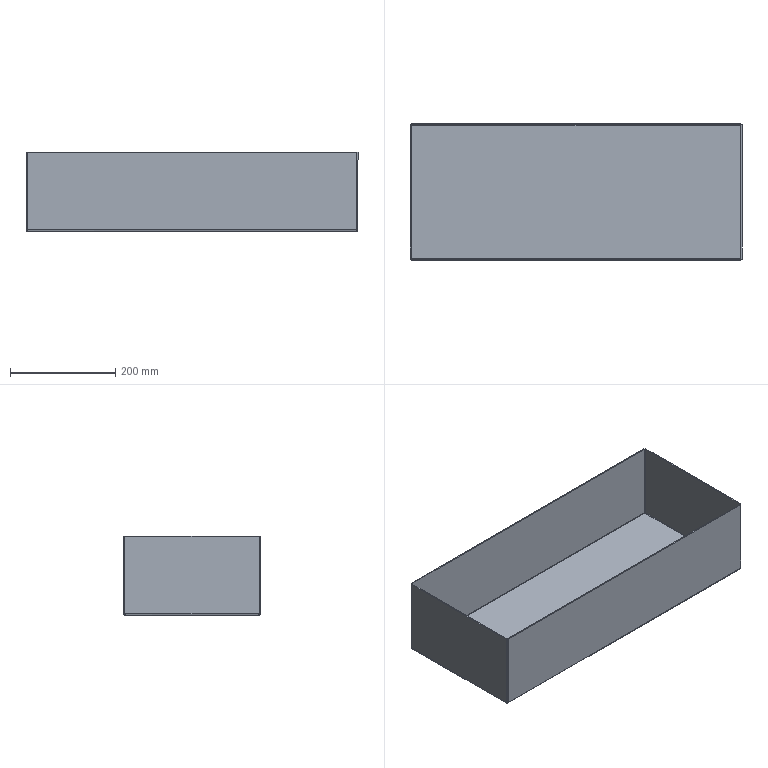Part | SolidWorks | features EdgeFlange 1, FlatPattern 1, SMBaseFlange 1, SheetMetal 1 | 1 solid | 38 faces | box 630 x 260 x 150 mm | volume 844986 mm3 | plane 22 | spline 8 | cylinder 8 | commonest cylinder face diameters 2 x4 6 x4
STEP:
#1=CARTESIAN_POINT('',(312.,127.,-2.));
#2=VERTEX_POINT('',#1);
#3=CARTESIAN_POINT('',(312.,-127.,-2.));
#4=VERTEX_POINT('',#3);
#5=CARTESIAN_POINT('',(312.,127.293,-2.));
#6=DIRECTION('',(0.,-1.,0.));
#7=VECTOR('',#6,1000.);
#8=LINE('',#5,#7);
#9=EDGE_CURVE('',#2,#4,#8,.T.);
#10=ORIENTED_EDGE('',*,*,#9,.T.);
#11=CARTESIAN_POINT('',(-312.,-127.,-2.));
#12=VERTEX_POINT('',#11);
#13=CARTESIAN_POINT('',(312.293,-127.,-2.));
#14=DIRECTION('',(-1.,0.,0.));
#15=VECTOR('',#14,1000.);
#16=LINE('',#13,#15);
#17=EDGE_CURVE('',#4,#12,#16,.T.);
#18=ORIENTED_EDGE('',*,*,#17,.T.);
#19=CARTESIAN_POINT('',(-312.,127.,-2.));
#20=VERTEX_POINT('',#19);
#21=CARTESIAN_POINT('',(-312.,-127.293,-2.));
#22=DIRECTION('',(0.,1.,0.));
#23=VECTOR('',#22,1000.);
#24=LINE('',#21,#23);
#25=EDGE_CURVE('',#12,#20,#24,.T.);
#26=ORIENTED_EDGE('',*,*,#25,.T.);
#27=CARTESIAN_POINT('',(-312.293,127.,-2.));
#28=DIRECTION('',(1.,0.,0.));
#29=VECTOR('',#28,1000.);
#30=LINE('',#27,#29);
#31=EDGE_CURVE('',#20,#2,#30,.T.);
#32=ORIENTED_EDGE('',*,*,#31,.T.);
#33=EDGE_LOOP('',(#10,#18,#26,#32));
#34=FACE_OUTER_BOUND('',#33,.T.);
#35=CARTESIAN_POINT('',(0.,0.,-2.));
#36=DIRECTION('',(0.,0.,1.));
#37=DIRECTION('',(1.,0.,0.));
#38=AXIS2_PLACEMENT_3D('',#35,#36,#37);
#39=PLANE('',#38);
#40=ADVANCED_FACE('',(#34),#39,.F.);
#41=CARTESIAN_POINT('',(312.,-127.,0.));
#42=VERTEX_POINT('',#41);
#43=CARTESIAN_POINT('',(-312.,-127.,0.));
#44=VERTEX_POINT('',#43);
#45=CARTESIAN_POINT('',(312.293,-127.,0.));
#46=DIRECTION('',(-1.,0.,0.));
#47=VECTOR('',#46,1000.);
#48=LINE('',#45,#47);
#49=EDGE_CURVE('',#42,#44,#48,.T.);
#50=ORIENTED_EDGE('',*,*,#49,.F.);
#51=CARTESIAN_POINT('',(312.,127.,0.));
#52=VERTEX_POINT('',#51);
#53=CARTESIAN_POINT('',(312.,127.293,0.));
#54=DIRECTION('',(0.,-1.,0.));
#55=VECTOR('',#54,1000.);
#56=LINE('',#53,#55);
#57=EDGE_CURVE('',#52,#42,#56,.T.);
#58=ORIENTED_EDGE('',*,*,#57,.F.);
#59=CARTESIAN_POINT('',(-312.,127.,0.));
#60=VERTEX_POINT('',#59);
#61=CARTESIAN_POINT('',(-312.293,127.,0.));
#62=DIRECTION('',(1.,0.,0.));
#63=VECTOR('',#62,1000.);
#64=LINE('',#61,#63);
#65=EDGE_CURVE('',#60,#52,#64,.T.);
#66=ORIENTED_EDGE('',*,*,#65,.F.);
#67=CARTESIAN_POINT('',(-312.,-127.293,0.));
#68=DIRECTION('',(0.,1.,0.));
#69=VECTOR('',#68,1000.);
#70=LINE('',#67,#69);
#71=EDGE_CURVE('',#44,#60,#70,.T.);
#72=ORIENTED_EDGE('',*,*,#71,.F.);
#73=EDGE_LOOP('',(#50,#58,#66,#72));
#74=FACE_OUTER_BOUND('',#73,.T.);
#75=CARTESIAN_POINT('',(0.,0.,0.));
#76=DIRECTION('',(0.,0.,1.));
#77=DIRECTION('',(1.,0.,0.));
#78=AXIS2_PLACEMENT_3D('',#75,#76,#77);
#79=PLANE('',#78);
#80=ADVANCED_FACE('',(#74),#79,.T.);
#81=CARTESIAN_POINT('',(-315.,127.293,1.));
#82=VERTEX_POINT('',#81);
#83=CARTESIAN_POINT('',(-313.,127.293,1.));
#84=VERTEX_POINT('',#83);
#85=CARTESIAN_POINT('',(-313.,127.293,1.));
#86=DIRECTION('',(1.,0.,0.));
#87=VECTOR('',#86,1000.);
#88=LINE('',#85,#87);
#89=EDGE_CURVE('',#82,#84,#88,.T.);
#90=ORIENTED_EDGE('',*,*,#89,.T.);
#91=CARTESIAN_POINT('',(-312.,127.,0.));
#92=CARTESIAN_POINT('',(-312.262,127.049,0.));
#93=CARTESIAN_POINT('',(-312.522,127.098,0.1078));
#94=CARTESIAN_POINT('',(-312.892,127.195,0.478));
#95=CARTESIAN_POINT('',(-313.,127.244,0.7382));
#96=CARTESIAN_POINT('',(-313.,127.293,1.));
#97=B_SPLINE_CURVE_WITH_KNOTS('',3,(#91,#92,#93,#94,#95,#96),.UNSPECIFIED.,.F.,.F.,(4,2,4),(0.,0.5,1.),.UNSPECIFIED.);
#98=EDGE_CURVE('',#60,#84,#97,.T.);
#99=ORIENTED_EDGE('',*,*,#98,.F.);
#100=CARTESIAN_POINT('',(-312.,127.,0.));
#101=DIRECTION('',(0.,0.,-1.));
#102=VECTOR('',#101,1000.);
#103=LINE('',#100,#102);
#104=EDGE_CURVE('',#60,#20,#103,.T.);
#105=ORIENTED_EDGE('',*,*,#104,.T.);
#106=CARTESIAN_POINT('',(-312.,127.,-2.));
#107=CARTESIAN_POINT('',(-312.393,127.024,-2.));
#108=CARTESIAN_POINT('',(-312.785,127.049,-1.922));
#109=CARTESIAN_POINT('',(-313.511,127.098,-1.621));
#110=CARTESIAN_POINT('',(-313.844,127.122,-1.399));
#111=CARTESIAN_POINT('',(-314.399,127.171,-0.8436));
#112=CARTESIAN_POINT('',(-314.621,127.195,-0.5109));
#113=CARTESIAN_POINT('',(-314.922,127.244,0.2148));
#114=CARTESIAN_POINT('',(-315.,127.268,0.6073));
#115=CARTESIAN_POINT('',(-315.,127.293,1.));
#116=B_SPLINE_CURVE_WITH_KNOTS('',3,(#106,#107,#108,#109,#110,#111,#112,#113,#114,#115),.UNSPECIFIED.,.F.,.F.,(4,2,2,2,4),(0.,0.25,0.5,0.75,1.),.UNSPECIFIED.);
#117=EDGE_CURVE('',#20,#82,#116,.T.);
#118=ORIENTED_EDGE('',*,*,#117,.T.);
#119=EDGE_LOOP('',(#90,#99,#105,#118));
#120=FACE_OUTER_BOUND('',#119,.T.);
#121=CARTESIAN_POINT('',(-312.,127.,-2.02));
#122=CARTESIAN_POINT('',(-312.395,127.024,-2.02));
#123=CARTESIAN_POINT('',(-312.79,127.049,-1.941));
#124=CARTESIAN_POINT('',(-313.521,127.098,-1.639));
#125=CARTESIAN_POINT('',(-313.856,127.122,-1.415));
#126=CARTESIAN_POINT('',(-314.415,127.171,-0.8559));
#127=CARTESIAN_POINT('',(-314.639,127.195,-0.5209));
#128=CARTESIAN_POINT('',(-314.941,127.244,0.2095));
#129=CARTESIAN_POINT('',(-315.02,127.268,0.6046));
#130=CARTESIAN_POINT('',(-315.02,127.293,1.));
#131=CARTESIAN_POINT('',(-312.,127.,-2.));
#132=CARTESIAN_POINT('',(-312.393,127.024,-2.));
#133=CARTESIAN_POINT('',(-312.785,127.049,-1.922));
#134=CARTESIAN_POINT('',(-313.511,127.098,-1.621));
#135=CARTESIAN_POINT('',(-313.844,127.122,-1.399));
#136=CARTESIAN_POINT('',(-314.399,127.171,-0.8436));
#137=CARTESIAN_POINT('',(-314.621,127.195,-0.5109));
#138=CARTESIAN_POINT('',(-314.922,127.244,0.2148));
#139=CARTESIAN_POINT('',(-315.,127.268,0.6072));
#140=CARTESIAN_POINT('',(-315.,127.293,1.));
#141=CARTESIAN_POINT('',(-312.,127.,0.));
#142=CARTESIAN_POINT('',(-312.131,127.024,0.));
#143=CARTESIAN_POINT('',(-312.262,127.049,0.02603));
#144=CARTESIAN_POINT('',(-312.504,127.098,0.1262));
#145=CARTESIAN_POINT('',(-312.615,127.122,0.2003));
#146=CARTESIAN_POINT('',(-312.8,127.171,0.3855));
#147=CARTESIAN_POINT('',(-312.874,127.195,0.4964));
#148=CARTESIAN_POINT('',(-312.974,127.244,0.7383));
#149=CARTESIAN_POINT('',(-313.,127.268,0.8691));
#150=CARTESIAN_POINT('',(-313.,127.293,1.));
#151=CARTESIAN_POINT('',(-312.,127.,0.0202));
#152=CARTESIAN_POINT('',(-312.128,127.024,0.0202));
#153=CARTESIAN_POINT('',(-312.256,127.049,0.0457));
#154=CARTESIAN_POINT('',(-312.493,127.098,0.1439));
#155=CARTESIAN_POINT('',(-312.602,127.122,0.2165));
#156=CARTESIAN_POINT('',(-312.784,127.171,0.3979));
#157=CARTESIAN_POINT('',(-312.856,127.195,0.5066));
#158=CARTESIAN_POINT('',(-312.954,127.244,0.7435));
#159=CARTESIAN_POINT('',(-312.98,127.268,0.8717));
#160=CARTESIAN_POINT('',(-312.98,127.293,1.));
#161=B_SPLINE_SURFACE_WITH_KNOTS('',1,3,((#121,#122,#123,#124,#125,#126,#127,#128,#129,#130),(#131,#132,#133,#134,#135,#136,#137,#138,#139,#140),(#141,#142,#143,#144,#145,#146,#147,#148,#149,#150),(#151,#152,#153,#154,#155,#156,#157,#158,#159,#160)),.UNSPECIFIED.,.F.,.F.,.F.,(2,1,1,2),(4,2,2,2,4),(-0.01,0.,1.,1.01),(0.,0.25,0.5,0.75,1.),.UNSPECIFIED.);
#162=ADVANCED_FACE('',(#120),#161,.F.);
#163=CARTESIAN_POINT('',(-313.,-127.293,1.));
#164=VERTEX_POINT('',#163);
#165=CARTESIAN_POINT('',(-313.,-127.293,1.));
#166=CARTESIAN_POINT('',(-313.,-127.244,0.7382));
#167=CARTESIAN_POINT('',(-312.892,-127.195,0.478));
#168=CARTESIAN_POINT('',(-312.522,-127.098,0.1078));
#169=CARTESIAN_POINT('',(-312.262,-127.049,0.));
#170=CARTESIAN_POINT('',(-312.,-127.,0.));
#171=B_SPLINE_CURVE_WITH_KNOTS('',3,(#165,#166,#167,#168,#169,#170),.UNSPECIFIED.,.F.,.F.,(4,2,4),(0.,0.5,1.),.UNSPECIFIED.);
#172=EDGE_CURVE('',#164,#44,#171,.T.);
#173=ORIENTED_EDGE('',*,*,#172,.F.);
#174=CARTESIAN_POINT('',(-315.,-127.293,1.));
#175=VERTEX_POINT('',#174);
#176=CARTESIAN_POINT('',(-313.,-127.293,1.));
#177=DIRECTION('',(1.,0.,0.));
#178=VECTOR('',#177,1000.);
#179=LINE('',#176,#178);
#180=EDGE_CURVE('',#175,#164,#179,.T.);
#181=ORIENTED_EDGE('',*,*,#180,.F.);
#182=CARTESIAN_POINT('',(-315.,-127.293,1.));
#183=CARTESIAN_POINT('',(-315.,-127.268,0.6073));
#184=CARTESIAN_POINT('',(-314.922,-127.244,0.2148));
#185=CARTESIAN_POINT('',(-314.621,-127.195,-0.5109));
#186=CARTESIAN_POINT('',(-314.399,-127.171,-0.8436));
#187=CARTESIAN_POINT('',(-313.844,-127.122,-1.399));
#188=CARTESIAN_POINT('',(-313.511,-127.098,-1.621));
#189=CARTESIAN_POINT('',(-312.785,-127.049,-1.922));
#190=CARTESIAN_POINT('',(-312.393,-127.024,-2.));
#191=CARTESIAN_POINT('',(-312.,-127.,-2.));
#192=B_SPLINE_CURVE_WITH_KNOTS('',3,(#182,#183,#184,#185,#186,#187,#188,#189,#190,#191),.UNSPECIFIED.,.F.,.F.,(4,2,2,2,4),(0.,0.25,0.5,0.75,1.),.UNSPECIFIED.);
#193=EDGE_CURVE('',#175,#12,#192,.T.);
#194=ORIENTED_EDGE('',*,*,#193,.T.);
#195=CARTESIAN_POINT('',(-312.,-127.,0.));
#196=DIRECTION('',(0.,0.,-1.));
#197=VECTOR('',#196,1000.);
#198=LINE('',#195,#197);
#199=EDGE_CURVE('',#44,#12,#198,.T.);
#200=ORIENTED_EDGE('',*,*,#199,.F.);
#201=EDGE_LOOP('',(#173,#181,#194,#200));
#202=FACE_OUTER_BOUND('',#201,.T.);
#203=CARTESIAN_POINT('',(-315.02,-127.293,1.));
#204=CARTESIAN_POINT('',(-315.02,-127.268,0.6046));
#205=CARTESIAN_POINT('',(-314.941,-127.244,0.2095));
#206=CARTESIAN_POINT('',(-314.639,-127.195,-0.5209));
#207=CARTESIAN_POINT('',(-314.415,-127.171,-0.8559));
#208=CARTESIAN_POINT('',(-313.856,-127.122,-1.415));
#209=CARTESIAN_POINT('',(-313.521,-127.098,-1.639));
#210=CARTESIAN_POINT('',(-312.79,-127.049,-1.941));
#211=CARTESIAN_POINT('',(-312.395,-127.024,-2.02));
#212=CARTESIAN_POINT('',(-312.,-127.,-2.02));
#213=CARTESIAN_POINT('',(-315.,-127.293,1.));
#214=CARTESIAN_POINT('',(-315.,-127.268,0.6072));
#215=CARTESIAN_POINT('',(-314.922,-127.244,0.2148));
#216=CARTESIAN_POINT('',(-314.621,-127.195,-0.5109));
#217=CARTESIAN_POINT('',(-314.399,-127.171,-0.8436));
#218=CARTESIAN_POINT('',(-313.844,-127.122,-1.399));
#219=CARTESIAN_POINT('',(-313.511,-127.098,-1.621));
#220=CARTESIAN_POINT('',(-312.785,-127.049,-1.922));
#221=CARTESIAN_POINT('',(-312.393,-127.024,-2.));
#222=CARTESIAN_POINT('',(-312.,-127.,-2.));
#223=CARTESIAN_POINT('',(-313.,-127.293,1.));
#224=CARTESIAN_POINT('',(-313.,-127.268,0.8691));
#225=CARTESIAN_POINT('',(-312.974,-127.244,0.7383));
#226=CARTESIAN_POINT('',(-312.874,-127.195,0.4964));
#227=CARTESIAN_POINT('',(-312.8,-127.171,0.3855));
#228=CARTESIAN_POINT('',(-312.615,-127.122,0.2003));
#229=CARTESIAN_POINT('',(-312.504,-127.098,0.1262));
#230=CARTESIAN_POINT('',(-312.262,-127.049,0.02603));
#231=CARTESIAN_POINT('',(-312.131,-127.024,0.));
#232=CARTESIAN_POINT('',(-312.,-127.,0.));
#233=CARTESIAN_POINT('',(-312.98,-127.293,1.));
#234=CARTESIAN_POINT('',(-312.98,-127.268,0.8717));
#235=CARTESIAN_POINT('',(-312.954,-127.244,0.7435));
#236=CARTESIAN_POINT('',(-312.856,-127.195,0.5066));
#237=CARTESIAN_POINT('',(-312.784,-127.171,0.3979));
#238=CARTESIAN_POINT('',(-312.602,-127.122,0.2165));
#239=CARTESIAN_POINT('',(-312.493,-127.098,0.1439));
#240=CARTESIAN_POINT('',(-312.256,-127.049,0.0457));
#241=CARTESIAN_POINT('',(-312.128,-127.024,0.0202));
#242=CARTESIAN_POINT('',(-312.,-127.,0.0202));
#243=B_SPLINE_SURFACE_WITH_KNOTS('',1,3,((#203,#204,#205,#206,#207,#208,#209,#210,#211,#212),(#213,#214,#215,#216,#217,#218,#219,#220,#221,#222),(#223,#224,#225,#226,#227,#228,#229,#230,#231,#232),(#233,#234,#235,#236,#237,#238,#239,#240,#241,#242)),.UNSPECIFIED.,.F.,.F.,.F.,(2,1,1,2),(4,2,2,2,4),(-0.01,0.,1.,1.01),(0.,0.25,0.5,0.75,1.),.UNSPECIFIED.);
#244=ADVANCED_FACE('',(#202),#243,.F.);
#245=ORIENTED_EDGE('',*,*,#25,.F.);
#246=ORIENTED_EDGE('',*,*,#193,.F.);
#247=CARTESIAN_POINT('',(-315.,130.,1.));
#248=DIRECTION('',(0.,1.,0.));
#249=VECTOR('',#248,1000.);
#250=LINE('',#247,#249);
#251=EDGE_CURVE('',#175,#82,#250,.T.);
#252=ORIENTED_EDGE('',*,*,#251,.T.);
#253=ORIENTED_EDGE('',*,*,#117,.F.);
#254=EDGE_LOOP('',(#245,#246,#252,#253));
#255=FACE_OUTER_BOUND('',#254,.T.);
#256=CARTESIAN_POINT('',(-312.,-127.293,1.));
#257=DIRECTION('',(0.,-1.,0.));
#258=DIRECTION('',(-1.,0.,0.));
#259=AXIS2_PLACEMENT_3D('',#256,#257,#258);
#260=CYLINDRICAL_SURFACE('',#259,3.);
#261=ADVANCED_FACE('',(#255),#260,.T.);
#262=ORIENTED_EDGE('',*,*,#71,.T.);
#263=ORIENTED_EDGE('',*,*,#98,.T.);
#264=CARTESIAN_POINT('',(-313.,130.,1.));
#265=DIRECTION('',(0.,-1.,0.));
#266=VECTOR('',#265,1000.);
#267=LINE('',#264,#266);
#268=EDGE_CURVE('',#84,#164,#267,.T.);
#269=ORIENTED_EDGE('',*,*,#268,.T.);
#270=ORIENTED_EDGE('',*,*,#172,.T.);
#271=EDGE_LOOP('',(#262,#263,#269,#270));
#272=FACE_OUTER_BOUND('',#271,.T.);
#273=CARTESIAN_POINT('',(-312.,-127.293,1.));
#274=DIRECTION('',(0.,-1.,0.));
#275=DIRECTION('',(-1.,0.,0.));
#276=AXIS2_PLACEMENT_3D('',#273,#274,#275);
#277=CYLINDRICAL_SURFACE('',#276,1.);
#278=ADVANCED_FACE('',(#272),#277,.F.);
#279=CARTESIAN_POINT('',(-315.,127.293,148.));
#280=VERTEX_POINT('',#279);
#281=CARTESIAN_POINT('',(-315.,127.293,0.));
#282=DIRECTION('',(0.,0.,1.));
#283=VECTOR('',#282,1000.);
#284=LINE('',#281,#283);
#285=EDGE_CURVE('',#82,#280,#284,.T.);
#286=ORIENTED_EDGE('',*,*,#285,.T.);
#287=CARTESIAN_POINT('',(-313.,127.293,148.));
#288=VERTEX_POINT('',#287);
#289=CARTESIAN_POINT('',(-313.,127.293,148.));
#290=DIRECTION('',(1.,0.,0.));
#291=VECTOR('',#290,1000.);
#292=LINE('',#289,#291);
#293=EDGE_CURVE('',#280,#288,#292,.T.);
#294=ORIENTED_EDGE('',*,*,#293,.T.);
#295=CARTESIAN_POINT('',(-313.,127.293,0.));
#296=DIRECTION('',(0.,0.,1.));
#297=VECTOR('',#296,1000.);
#298=LINE('',#295,#297);
#299=EDGE_CURVE('',#84,#288,#298,.T.);
#300=ORIENTED_EDGE('',*,*,#299,.F.);
#301=ORIENTED_EDGE('',*,*,#89,.F.);
#302=EDGE_LOOP('',(#286,#294,#300,#301));
#303=FACE_OUTER_BOUND('',#302,.T.);
#304=CARTESIAN_POINT('',(-313.,127.293,0.));
#305=DIRECTION('',(0.,1.,0.));
#306=DIRECTION('',(0.,0.,1.));
#307=AXIS2_PLACEMENT_3D('',#304,#305,#306);
#308=PLANE('',#307);
#309=ADVANCED_FACE('',(#303),#308,.T.);
#310=ORIENTED_EDGE('',*,*,#251,.F.);
#311=CARTESIAN_POINT('',(-315.,-127.293,148.));
#312=VERTEX_POINT('',#311);
#313=CARTESIAN_POINT('',(-315.,-127.293,0.));
#314=DIRECTION('',(0.,0.,1.));
#315=VECTOR('',#314,1000.);
#316=LINE('',#313,#315);
#317=EDGE_CURVE('',#175,#312,#316,.T.);
#318=ORIENTED_EDGE('',*,*,#317,.T.);
#319=CARTESIAN_POINT('',(-315.,0.,148.));
#320=DIRECTION('',(0.,1.,0.));
#321=VECTOR('',#320,1000.);
#322=LINE('',#319,#321);
#323=EDGE_CURVE('',#312,#280,#322,.T.);
#324=ORIENTED_EDGE('',*,*,#323,.T.);
#325=ORIENTED_EDGE('',*,*,#285,.F.);
#326=EDGE_LOOP('',(#310,#318,#324,#325));
#327=FACE_OUTER_BOUND('',#326,.T.);
#328=CARTESIAN_POINT('',(-315.,0.,0.));
#329=DIRECTION('',(1.,0.,0.));
#330=DIRECTION('',(0.,0.,-1.));
#331=AXIS2_PLACEMENT_3D('',#328,#329,#330);
#332=PLANE('',#331);
#333=ADVANCED_FACE('',(#327),#332,.F.);
#334=CARTESIAN_POINT('',(-313.,-127.293,148.));
#335=VERTEX_POINT('',#334);
#336=CARTESIAN_POINT('',(-313.,-127.293,0.));
#337=DIRECTION('',(0.,0.,1.));
#338=VECTOR('',#337,1000.);
#339=LINE('',#336,#338);
#340=EDGE_CURVE('',#164,#335,#339,.T.);
#341=ORIENTED_EDGE('',*,*,#340,.F.);
#342=ORIENTED_EDGE('',*,*,#268,.F.);
#343=ORIENTED_EDGE('',*,*,#299,.T.);
#344=CARTESIAN_POINT('',(-313.,130.,148.));
#345=DIRECTION('',(0.,1.,0.));
#346=VECTOR('',#345,1000.);
#347=LINE('',#344,#346);
#348=EDGE_CURVE('',#335,#288,#347,.T.);
#349=ORIENTED_EDGE('',*,*,#348,.F.);
#350=EDGE_LOOP('',(#341,#342,#343,#349));
#351=FACE_OUTER_BOUND('',#350,.T.);
#352=CARTESIAN_POINT('',(-313.,0.,0.));
#353=DIRECTION('',(1.,0.,0.));
#354=DIRECTION('',(0.,0.,-1.));
#355=AXIS2_PLACEMENT_3D('',#352,#353,#354);
#356=PLANE('',#355);
#357=ADVANCED_FACE('',(#351),#356,.T.);
#358=ORIENTED_EDGE('',*,*,#323,.F.);
#359=CARTESIAN_POINT('',(-315.,-127.293,148.));
#360=DIRECTION('',(1.,0.,0.));
#361=VECTOR('',#360,1000.);
#362=LINE('',#359,#361);
#363=EDGE_CURVE('',#312,#335,#362,.T.);
#364=ORIENTED_EDGE('',*,*,#363,.T.);
#365=ORIENTED_EDGE('',*,*,#348,.T.);
#366=ORIENTED_EDGE('',*,*,#293,.F.);
#367=EDGE_LOOP('',(#358,#364,#365,#366));
#368=FACE_OUTER_BOUND('',#367,.T.);
#369=CARTESIAN_POINT('',(-315.,130.,148.));
#370=DIRECTION('',(0.,0.,-1.));
#371=DIRECTION('',(-1.,0.,0.));
#372=AXIS2_PLACEMENT_3D('',#369,#370,#371);
#373=PLANE('',#372);
#374=ADVANCED_FACE('',(#368),#373,.F.);
#375=ORIENTED_EDGE('',*,*,#363,.F.);
#376=ORIENTED_EDGE('',*,*,#317,.F.);
#377=ORIENTED_EDGE('',*,*,#180,.T.);
#378=ORIENTED_EDGE('',*,*,#340,.T.);
#379=EDGE_LOOP('',(#375,#376,#377,#378));
#380=FACE_OUTER_BOUND('',#379,.T.);
#381=CARTESIAN_POINT('',(-313.,-127.293,0.));
#382=DIRECTION('',(0.,1.,0.));
#383=DIRECTION('',(0.,0.,1.));
#384=AXIS2_PLACEMENT_3D('',#381,#382,#383);
#385=PLANE('',#384);
#386=ADVANCED_FACE('',(#380),#385,.F.);
#387=CARTESIAN_POINT('',(312.293,130.,1.));
#388=VERTEX_POINT('',#387);
#389=CARTESIAN_POINT('',(312.293,128.,1.));
#390=VERTEX_POINT('',#389);
#391=CARTESIAN_POINT('',(312.293,128.,1.));
#392=DIRECTION('',(0.,-1.,0.));
#393=VECTOR('',#392,1000.);
#394=LINE('',#391,#393);
#395=EDGE_CURVE('',#388,#390,#394,.T.);
#396=ORIENTED_EDGE('',*,*,#395,.T.);
#397=CARTESIAN_POINT('',(312.,127.,0.));
#398=CARTESIAN_POINT('',(312.049,127.262,0.));
#399=CARTESIAN_POINT('',(312.098,127.522,0.1078));
#400=CARTESIAN_POINT('',(312.195,127.892,0.478));
#401=CARTESIAN_POINT('',(312.244,128.,0.7382));
#402=CARTESIAN_POINT('',(312.293,128.,1.));
#403=B_SPLINE_CURVE_WITH_KNOTS('',3,(#397,#398,#399,#400,#401,#402),.UNSPECIFIED.,.F.,.F.,(4,2,4),(0.,0.5,1.),.UNSPECIFIED.);
#404=EDGE_CURVE('',#52,#390,#403,.T.);
#405=ORIENTED_EDGE('',*,*,#404,.F.);
#406=CARTESIAN_POINT('',(312.,127.,0.));
#407=DIRECTION('',(0.,0.,-1.));
#408=VECTOR('',#407,1000.);
#409=LINE('',#406,#408);
#410=EDGE_CURVE('',#52,#2,#409,.T.);
#411=ORIENTED_EDGE('',*,*,#410,.T.);
#412=CARTESIAN_POINT('',(312.,127.,-2.));
#413=CARTESIAN_POINT('',(312.024,127.393,-2.));
#414=CARTESIAN_POINT('',(312.049,127.785,-1.922));
#415=CARTESIAN_POINT('',(312.098,128.511,-1.621));
#416=CARTESIAN_POINT('',(312.122,128.844,-1.399));
#417=CARTESIAN_POINT('',(312.171,129.399,-0.8436));
#418=CARTESIAN_POINT('',(312.195,129.621,-0.5109));
#419=CARTESIAN_POINT('',(312.244,129.922,0.2148));
#420=CARTESIAN_POINT('',(312.268,130.,0.6073));
#421=CARTESIAN_POINT('',(312.293,130.,1.));
#422=B_SPLINE_CURVE_WITH_KNOTS('',3,(#412,#413,#414,#415,#416,#417,#418,#419,#420,#421),.UNSPECIFIED.,.F.,.F.,(4,2,2,2,4),(0.,0.25,0.5,0.75,1.),.UNSPECIFIED.);
#423=EDGE_CURVE('',#2,#388,#422,.T.);
#424=ORIENTED_EDGE('',*,*,#423,.T.);
#425=EDGE_LOOP('',(#396,#405,#411,#424));
#426=FACE_OUTER_BOUND('',#425,.T.);
#427=CARTESIAN_POINT('',(312.,127.,-2.02));
#428=CARTESIAN_POINT('',(312.024,127.395,-2.02));
#429=CARTESIAN_POINT('',(312.049,127.79,-1.941));
#430=CARTESIAN_POINT('',(312.098,128.521,-1.639));
#431=CARTESIAN_POINT('',(312.122,128.856,-1.415));
#432=CARTESIAN_POINT('',(312.171,129.415,-0.8559));
#433=CARTESIAN_POINT('',(312.195,129.639,-0.5209));
#434=CARTESIAN_POINT('',(312.244,129.941,0.2095));
#435=CARTESIAN_POINT('',(312.268,130.02,0.6046));
#436=CARTESIAN_POINT('',(312.293,130.02,1.));
#437=CARTESIAN_POINT('',(312.,127.,-2.));
#438=CARTESIAN_POINT('',(312.024,127.393,-2.));
#439=CARTESIAN_POINT('',(312.049,127.785,-1.922));
#440=CARTESIAN_POINT('',(312.098,128.511,-1.621));
#441=CARTESIAN_POINT('',(312.122,128.844,-1.399));
#442=CARTESIAN_POINT('',(312.171,129.399,-0.8436));
#443=CARTESIAN_POINT('',(312.195,129.621,-0.5109));
#444=CARTESIAN_POINT('',(312.244,129.922,0.2148));
#445=CARTESIAN_POINT('',(312.268,130.,0.6072));
#446=CARTESIAN_POINT('',(312.293,130.,1.));
#447=CARTESIAN_POINT('',(312.,127.,0.));
#448=CARTESIAN_POINT('',(312.024,127.131,0.));
#449=CARTESIAN_POINT('',(312.049,127.262,0.02603));
#450=CARTESIAN_POINT('',(312.098,127.504,0.1262));
#451=CARTESIAN_POINT('',(312.122,127.615,0.2003));
#452=CARTESIAN_POINT('',(312.171,127.8,0.3855));
#453=CARTESIAN_POINT('',(312.195,127.874,0.4964));
#454=CARTESIAN_POINT('',(312.244,127.974,0.7383));
#455=CARTESIAN_POINT('',(312.268,128.,0.8691));
#456=CARTESIAN_POINT('',(312.293,128.,1.));
#457=CARTESIAN_POINT('',(312.,127.,0.0202));
#458=CARTESIAN_POINT('',(312.024,127.128,0.0202));
#459=CARTESIAN_POINT('',(312.049,127.256,0.0457));
#460=CARTESIAN_POINT('',(312.098,127.493,0.1439));
#461=CARTESIAN_POINT('',(312.122,127.602,0.2165));
#462=CARTESIAN_POINT('',(312.171,127.784,0.3979));
#463=CARTESIAN_POINT('',(312.195,127.856,0.5066));
#464=CARTESIAN_POINT('',(312.244,127.954,0.7435));
#465=CARTESIAN_POINT('',(312.268,127.98,0.8717));
#466=CARTESIAN_POINT('',(312.293,127.98,1.));
#467=B_SPLINE_SURFACE_WITH_KNOTS('',1,3,((#427,#428,#429,#430,#431,#432,#433,#434,#435,#436),(#437,#438,#439,#440,#441,#442,#443,#444,#445,#446),(#447,#448,#449,#450,#451,#452,#453,#454,#455,#456),(#457,#458,#459,#460,#461,#462,#463,#464,#465,#466)),.UNSPECIFIED.,.F.,.F.,.F.,(2,1,1,2),(4,2,2,2,4),(-0.01,0.,1.,1.01),(0.,0.25,0.5,0.75,1.),.UNSPECIFIED.);
#468=ADVANCED_FACE('',(#426),#467,.F.);
#469=CARTESIAN_POINT('',(-312.293,128.,1.));
#470=VERTEX_POINT('',#469);
#471=CARTESIAN_POINT('',(-312.293,128.,1.));
#472=CARTESIAN_POINT('',(-312.244,128.,0.7382));
#473=CARTESIAN_POINT('',(-312.195,127.892,0.478));
#474=CARTESIAN_POINT('',(-312.098,127.522,0.1078));
#475=CARTESIAN_POINT('',(-312.049,127.262,0.));
#476=CARTESIAN_POINT('',(-312.,127.,0.));
#477=B_SPLINE_CURVE_WITH_KNOTS('',3,(#471,#472,#473,#474,#475,#476),.UNSPECIFIED.,.F.,.F.,(4,2,4),(0.,0.5,1.),.UNSPECIFIED.);
#478=EDGE_CURVE('',#470,#60,#477,.T.);
#479=ORIENTED_EDGE('',*,*,#478,.F.);
#480=CARTESIAN_POINT('',(-312.293,130.,1.));
#481=VERTEX_POINT('',#480);
#482=CARTESIAN_POINT('',(-312.293,128.,1.));
#483=DIRECTION('',(0.,-1.,0.));
#484=VECTOR('',#483,1000.);
#485=LINE('',#482,#484);
#486=EDGE_CURVE('',#481,#470,#485,.T.);
#487=ORIENTED_EDGE('',*,*,#486,.F.);
#488=CARTESIAN_POINT('',(-312.293,130.,1.));
#489=CARTESIAN_POINT('',(-312.268,130.,0.6073));
#490=CARTESIAN_POINT('',(-312.244,129.922,0.2148));
#491=CARTESIAN_POINT('',(-312.195,129.621,-0.5109));
#492=CARTESIAN_POINT('',(-312.171,129.399,-0.8436));
#493=CARTESIAN_POINT('',(-312.122,128.844,-1.399));
#494=CARTESIAN_POINT('',(-312.098,128.511,-1.621));
#495=CARTESIAN_POINT('',(-312.049,127.785,-1.922));
#496=CARTESIAN_POINT('',(-312.024,127.393,-2.));
#497=CARTESIAN_POINT('',(-312.,127.,-2.));
#498=B_SPLINE_CURVE_WITH_KNOTS('',3,(#488,#489,#490,#491,#492,#493,#494,#495,#496,#497),.UNSPECIFIED.,.F.,.F.,(4,2,2,2,4),(0.,0.25,0.5,0.75,1.),.UNSPECIFIED.);
#499=EDGE_CURVE('',#481,#20,#498,.T.);
#500=ORIENTED_EDGE('',*,*,#499,.T.);
#501=ORIENTED_EDGE('',*,*,#104,.F.);
#502=EDGE_LOOP('',(#479,#487,#500,#501));
#503=FACE_OUTER_BOUND('',#502,.T.);
#504=CARTESIAN_POINT('',(-312.293,130.02,1.));
#505=CARTESIAN_POINT('',(-312.268,130.02,0.6046));
#506=CARTESIAN_POINT('',(-312.244,129.941,0.2095));
#507=CARTESIAN_POINT('',(-312.195,129.639,-0.5209));
#508=CARTESIAN_POINT('',(-312.171,129.415,-0.8559));
#509=CARTESIAN_POINT('',(-312.122,128.856,-1.415));
#510=CARTESIAN_POINT('',(-312.098,128.521,-1.639));
#511=CARTESIAN_POINT('',(-312.049,127.79,-1.941));
#512=CARTESIAN_POINT('',(-312.024,127.395,-2.02));
#513=CARTESIAN_POINT('',(-312.,127.,-2.02));
#514=CARTESIAN_POINT('',(-312.293,130.,1.));
#515=CARTESIAN_POINT('',(-312.268,130.,0.6072));
#516=CARTESIAN_POINT('',(-312.244,129.922,0.2148));
#517=CARTESIAN_POINT('',(-312.195,129.621,-0.5109));
#518=CARTESIAN_POINT('',(-312.171,129.399,-0.8436));
#519=CARTESIAN_POINT('',(-312.122,128.844,-1.399));
#520=CARTESIAN_POINT('',(-312.098,128.511,-1.621));
#521=CARTESIAN_POINT('',(-312.049,127.785,-1.922));
#522=CARTESIAN_POINT('',(-312.024,127.393,-2.));
#523=CARTESIAN_POINT('',(-312.,127.,-2.));
#524=CARTESIAN_POINT('',(-312.293,128.,1.));
#525=CARTESIAN_POINT('',(-312.268,128.,0.8691));
#526=CARTESIAN_POINT('',(-312.244,127.974,0.7383));
#527=CARTESIAN_POINT('',(-312.195,127.874,0.4964));
#528=CARTESIAN_POINT('',(-312.171,127.8,0.3855));
#529=CARTESIAN_POINT('',(-312.122,127.615,0.2003));
#530=CARTESIAN_POINT('',(-312.098,127.504,0.1262));
#531=CARTESIAN_POINT('',(-312.049,127.262,0.02603));
#532=CARTESIAN_POINT('',(-312.024,127.131,0.));
#533=CARTESIAN_POINT('',(-312.,127.,0.));
#534=CARTESIAN_POINT('',(-312.293,127.98,1.));
#535=CARTESIAN_POINT('',(-312.268,127.98,0.8717));
#536=CARTESIAN_POINT('',(-312.244,127.954,0.7435));
#537=CARTESIAN_POINT('',(-312.195,127.856,0.5066));
#538=CARTESIAN_POINT('',(-312.171,127.784,0.3979));
#539=CARTESIAN_POINT('',(-312.122,127.602,0.2165));
#540=CARTESIAN_POINT('',(-312.098,127.493,0.1439));
#541=CARTESIAN_POINT('',(-312.049,127.256,0.0457));
#542=CARTESIAN_POINT('',(-312.024,127.128,0.0202));
#543=CARTESIAN_POINT('',(-312.,127.,0.0202));
#544=B_SPLINE_SURFACE_WITH_KNOTS('',1,3,((#504,#505,#506,#507,#508,#509,#510,#511,#512,#513),(#514,#515,#516,#517,#518,#519,#520,#521,#522,#523),(#524,#525,#526,#527,#528,#529,#530,#531,#532,#533),(#534,#535,#536,#537,#538,#539,#540,#541,#542,#543)),.UNSPECIFIED.,.F.,.F.,.F.,(2,1,1,2),(4,2,2,2,4),(-0.01,0.,1.,1.01),(0.,0.25,0.5,0.75,1.),.UNSPECIFIED.);
#545=ADVANCED_FACE('',(#503),#544,.F.);
#546=ORIENTED_EDGE('',*,*,#31,.F.);
#547=ORIENTED_EDGE('',*,*,#499,.F.);
#548=CARTESIAN_POINT('',(315.,130.,1.));
#549=DIRECTION('',(1.,0.,0.));
#550=VECTOR('',#549,1000.);
#551=LINE('',#548,#550);
#552=EDGE_CURVE('',#481,#388,#551,.T.);
#553=ORIENTED_EDGE('',*,*,#552,.T.);
#554=ORIENTED_EDGE('',*,*,#423,.F.);
#555=EDGE_LOOP('',(#546,#547,#553,#554));
#556=FACE_OUTER_BOUND('',#555,.T.);
#557=CARTESIAN_POINT('',(-312.293,127.,1.));
#558=DIRECTION('',(-1.,0.,0.));
#559=DIRECTION('',(0.,1.,0.));
#560=AXIS2_PLACEMENT_3D('',#557,#558,#559);
#561=CYLINDRICAL_SURFACE('',#560,3.);
#562=ADVANCED_FACE('',(#556),#561,.T.);
#563=ORIENTED_EDGE('',*,*,#65,.T.);
#564=ORIENTED_EDGE('',*,*,#404,.T.);
#565=CARTESIAN_POINT('',(315.,128.,1.));
#566=DIRECTION('',(-1.,0.,0.));
#567=VECTOR('',#566,1000.);
#568=LINE('',#565,#567);
#569=EDGE_CURVE('',#390,#470,#568,.T.);
#570=ORIENTED_EDGE('',*,*,#569,.T.);
#571=ORIENTED_EDGE('',*,*,#478,.T.);
#572=EDGE_LOOP('',(#563,#564,#570,#571));
#573=FACE_OUTER_BOUND('',#572,.T.);
#574=CARTESIAN_POINT('',(-312.293,127.,1.));
#575=DIRECTION('',(-1.,0.,0.));
#576=DIRECTION('',(0.,1.,0.));
#577=AXIS2_PLACEMENT_3D('',#574,#575,#576);
#578=CYLINDRICAL_SURFACE('',#577,1.);
#579=ADVANCED_FACE('',(#573),#578,.F.);
#580=CARTESIAN_POINT('',(312.293,130.,148.));
#581=VERTEX_POINT('',#580);
#582=CARTESIAN_POINT('',(312.293,130.,0.));
#583=DIRECTION('',(0.,0.,1.));
#584=VECTOR('',#583,1000.);
#585=LINE('',#582,#584);
#586=EDGE_CURVE('',#388,#581,#585,.T.);
#587=ORIENTED_EDGE('',*,*,#586,.T.);
#588=CARTESIAN_POINT('',(312.293,128.,148.));
#589=VERTEX_POINT('',#588);
#590=CARTESIAN_POINT('',(312.293,128.,148.));
#591=DIRECTION('',(0.,-1.,0.));
#592=VECTOR('',#591,1000.);
#593=LINE('',#590,#592);
#594=EDGE_CURVE('',#581,#589,#593,.T.);
#595=ORIENTED_EDGE('',*,*,#594,.T.);
#596=CARTESIAN_POINT('',(312.293,128.,0.));
#597=DIRECTION('',(0.,0.,1.));
#598=VECTOR('',#597,1000.);
#599=LINE('',#596,#598);
#600=EDGE_CURVE('',#390,#589,#599,.T.);
#601=ORIENTED_EDGE('',*,*,#600,.F.);
#602=ORIENTED_EDGE('',*,*,#395,.F.);
#603=EDGE_LOOP('',(#587,#595,#601,#602));
#604=FACE_OUTER_BOUND('',#603,.T.);
#605=CARTESIAN_POINT('',(312.293,128.,0.));
#606=DIRECTION('',(1.,0.,0.));
#607=DIRECTION('',(0.,0.,-1.));
#608=AXIS2_PLACEMENT_3D('',#605,#606,#607);
#609=PLANE('',#608);
#610=ADVANCED_FACE('',(#604),#609,.T.);
#611=ORIENTED_EDGE('',*,*,#552,.F.);
#612=CARTESIAN_POINT('',(-312.293,130.,148.));
#613=VERTEX_POINT('',#612);
#614=CARTESIAN_POINT('',(-312.293,130.,0.));
#615=DIRECTION('',(0.,0.,1.));
#616=VECTOR('',#615,1000.);
#617=LINE('',#614,#616);
#618=EDGE_CURVE('',#481,#613,#617,.T.);
#619=ORIENTED_EDGE('',*,*,#618,.T.);
#620=CARTESIAN_POINT('',(0.,130.,148.));
#621=DIRECTION('',(1.,0.,0.));
#622=VECTOR('',#621,1000.);
#623=LINE('',#620,#622);
#624=EDGE_CURVE('',#613,#581,#623,.T.);
#625=ORIENTED_EDGE('',*,*,#624,.T.);
#626=ORIENTED_EDGE('',*,*,#586,.F.);
#627=EDGE_LOOP('',(#611,#619,#625,#626));
#628=FACE_OUTER_BOUND('',#627,.T.);
#629=CARTESIAN_POINT('',(0.,130.,0.));
#630=DIRECTION('',(0.,-1.,0.));
#631=DIRECTION('',(0.,0.,-1.));
#632=AXIS2_PLACEMENT_3D('',#629,#630,#631);
#633=PLANE('',#632);
#634=ADVANCED_FACE('',(#628),#633,.F.);
#635=CARTESIAN_POINT('',(-312.293,128.,148.));
#636=VERTEX_POINT('',#635);
#637=CARTESIAN_POINT('',(-312.293,128.,0.));
#638=DIRECTION('',(0.,0.,1.));
#639=VECTOR('',#638,1000.);
#640=LINE('',#637,#639);
#641=EDGE_CURVE('',#470,#636,#640,.T.);
#642=ORIENTED_EDGE('',*,*,#641,.F.);
#643=ORIENTED_EDGE('',*,*,#569,.F.);
#644=ORIENTED_EDGE('',*,*,#600,.T.);
#645=CARTESIAN_POINT('',(315.,128.,148.));
#646=DIRECTION('',(1.,0.,0.));
#647=VECTOR('',#646,1000.);
#648=LINE('',#645,#647);
#649=EDGE_CURVE('',#636,#589,#648,.T.);
#650=ORIENTED_EDGE('',*,*,#649,.F.);
#651=EDGE_LOOP('',(#642,#643,#644,#650));
#652=FACE_OUTER_BOUND('',#651,.T.);
#653=CARTESIAN_POINT('',(0.,128.,0.));
#654=DIRECTION('',(0.,-1.,0.));
#655=DIRECTION('',(0.,0.,-1.));
#656=AXIS2_PLACEMENT_3D('',#653,#654,#655);
#657=PLANE('',#656);
#658=ADVANCED_FACE('',(#652),#657,.T.);
#659=ORIENTED_EDGE('',*,*,#624,.F.);
#660=CARTESIAN_POINT('',(-312.293,130.,148.));
#661=DIRECTION('',(0.,-1.,0.));
#662=VECTOR('',#661,1000.);
#663=LINE('',#660,#662);
#664=EDGE_CURVE('',#613,#636,#663,.T.);
#665=ORIENTED_EDGE('',*,*,#664,.T.);
#666=ORIENTED_EDGE('',*,*,#649,.T.);
#667=ORIENTED_EDGE('',*,*,#594,.F.);
#668=EDGE_LOOP('',(#659,#665,#666,#667));
#669=FACE_OUTER_BOUND('',#668,.T.);
#670=CARTESIAN_POINT('',(315.,130.,148.));
#671=DIRECTION('',(0.,0.,-1.));
#672=DIRECTION('',(0.,1.,0.));
#673=AXIS2_PLACEMENT_3D('',#670,#671,#672);
#674=PLANE('',#673);
#675=ADVANCED_FACE('',(#669),#674,.F.);
#676=ORIENTED_EDGE('',*,*,#664,.F.);
#677=ORIENTED_EDGE('',*,*,#618,.F.);
#678=ORIENTED_EDGE('',*,*,#486,.T.);
#679=ORIENTED_EDGE('',*,*,#641,.T.);
#680=EDGE_LOOP('',(#676,#677,#678,#679));
#681=FACE_OUTER_BOUND('',#680,.T.);
#682=CARTESIAN_POINT('',(-312.293,128.,0.));
#683=DIRECTION('',(1.,0.,0.));
#684=DIRECTION('',(0.,0.,-1.));
#685=AXIS2_PLACEMENT_3D('',#682,#683,#684);
#686=PLANE('',#685);
#687=ADVANCED_FACE('',(#681),#686,.F.);
#688=CARTESIAN_POINT('',(-312.293,-130.,1.));
#689=VERTEX_POINT('',#688);
#690=CARTESIAN_POINT('',(-312.293,-128.,1.));
#691=VERTEX_POINT('',#690);
#692=CARTESIAN_POINT('',(-312.293,-128.,1.));
#693=DIRECTION('',(0.,1.,0.));
#694=VECTOR('',#693,1000.);
#695=LINE('',#692,#694);
#696=EDGE_CURVE('',#689,#691,#695,.T.);
#697=ORIENTED_EDGE('',*,*,#696,.T.);
#698=CARTESIAN_POINT('',(-312.,-127.,0.));
#699=CARTESIAN_POINT('',(-312.049,-127.262,0.));
#700=CARTESIAN_POINT('',(-312.098,-127.522,0.1078));
#701=CARTESIAN_POINT('',(-312.195,-127.892,0.478));
#702=CARTESIAN_POINT('',(-312.244,-128.,0.7382));
#703=CARTESIAN_POINT('',(-312.293,-128.,1.));
#704=B_SPLINE_CURVE_WITH_KNOTS('',3,(#698,#699,#700,#701,#702,#703),.UNSPECIFIED.,.F.,.F.,(4,2,4),(0.,0.5,1.),.UNSPECIFIED.);
#705=EDGE_CURVE('',#44,#691,#704,.T.);
#706=ORIENTED_EDGE('',*,*,#705,.F.);
#707=ORIENTED_EDGE('',*,*,#199,.T.);
#708=CARTESIAN_POINT('',(-312.,-127.,-2.));
#709=CARTESIAN_POINT('',(-312.024,-127.393,-2.));
#710=CARTESIAN_POINT('',(-312.049,-127.785,-1.922));
#711=CARTESIAN_POINT('',(-312.098,-128.511,-1.621));
#712=CARTESIAN_POINT('',(-312.122,-128.844,-1.399));
#713=CARTESIAN_POINT('',(-312.171,-129.399,-0.8436));
#714=CARTESIAN_POINT('',(-312.195,-129.621,-0.5109));
#715=CARTESIAN_POINT('',(-312.244,-129.922,0.2148));
#716=CARTESIAN_POINT('',(-312.268,-130.,0.6073));
#717=CARTESIAN_POINT('',(-312.293,-130.,1.));
#718=B_SPLINE_CURVE_WITH_KNOTS('',3,(#708,#709,#710,#711,#712,#713,#714,#715,#716,#717),.UNSPECIFIED.,.F.,.F.,(4,2,2,2,4),(0.,0.25,0.5,0.75,1.),.UNSPECIFIED.);
#719=EDGE_CURVE('',#12,#689,#718,.T.);
#720=ORIENTED_EDGE('',*,*,#719,.T.);
#721=EDGE_LOOP('',(#697,#706,#707,#720));
#722=FACE_OUTER_BOUND('',#721,.T.);
#723=CARTESIAN_POINT('',(-312.,-127.,-2.02));
#724=CARTESIAN_POINT('',(-312.024,-127.395,-2.02));
#725=CARTESIAN_POINT('',(-312.049,-127.79,-1.941));
#726=CARTESIAN_POINT('',(-312.098,-128.521,-1.639));
#727=CARTESIAN_POINT('',(-312.122,-128.856,-1.415));
#728=CARTESIAN_POINT('',(-312.171,-129.415,-0.8559));
#729=CARTESIAN_POINT('',(-312.195,-129.639,-0.5209));
#730=CARTESIAN_POINT('',(-312.244,-129.941,0.2095));
#731=CARTESIAN_POINT('',(-312.268,-130.02,0.6046));
#732=CARTESIAN_POINT('',(-312.293,-130.02,1.));
#733=CARTESIAN_POINT('',(-312.,-127.,-2.));
#734=CARTESIAN_POINT('',(-312.024,-127.393,-2.));
#735=CARTESIAN_POINT('',(-312.049,-127.785,-1.922));
#736=CARTESIAN_POINT('',(-312.098,-128.511,-1.621));
#737=CARTESIAN_POINT('',(-312.122,-128.844,-1.399));
#738=CARTESIAN_POINT('',(-312.171,-129.399,-0.8436));
#739=CARTESIAN_POINT('',(-312.195,-129.621,-0.5109));
#740=CARTESIAN_POINT('',(-312.244,-129.922,0.2148));
#741=CARTESIAN_POINT('',(-312.268,-130.,0.6072));
#742=CARTESIAN_POINT('',(-312.293,-130.,1.));
#743=CARTESIAN_POINT('',(-312.,-127.,0.));
#744=CARTESIAN_POINT('',(-312.024,-127.131,0.));
#745=CARTESIAN_POINT('',(-312.049,-127.262,0.02603));
#746=CARTESIAN_POINT('',(-312.098,-127.504,0.1262));
#747=CARTESIAN_POINT('',(-312.122,-127.615,0.2003));
#748=CARTESIAN_POINT('',(-312.171,-127.8,0.3855));
#749=CARTESIAN_POINT('',(-312.195,-127.874,0.4964));
#750=CARTESIAN_POINT('',(-312.244,-127.974,0.7383));
#751=CARTESIAN_POINT('',(-312.268,-128.,0.8691));
#752=CARTESIAN_POINT('',(-312.293,-128.,1.));
#753=CARTESIAN_POINT('',(-312.,-127.,0.0202));
#754=CARTESIAN_POINT('',(-312.024,-127.128,0.0202));
#755=CARTESIAN_POINT('',(-312.049,-127.256,0.0457));
#756=CARTESIAN_POINT('',(-312.098,-127.493,0.1439));
#757=CARTESIAN_POINT('',(-312.122,-127.602,0.2165));
#758=CARTESIAN_POINT('',(-312.171,-127.784,0.3979));
#759=CARTESIAN_POINT('',(-312.195,-127.856,0.5066));
#760=CARTESIAN_POINT('',(-312.244,-127.954,0.7435));
#761=CARTESIAN_POINT('',(-312.268,-127.98,0.8717));
#762=CARTESIAN_POINT('',(-312.293,-127.98,1.));
#763=B_SPLINE_SURFACE_WITH_KNOTS('',1,3,((#723,#724,#725,#726,#727,#728,#729,#730,#731,#732),(#733,#734,#735,#736,#737,#738,#739,#740,#741,#742),(#743,#744,#745,#746,#747,#748,#749,#750,#751,#752),(#753,#754,#755,#756,#757,#758,#759,#760,#761,#762)),.UNSPECIFIED.,.F.,.F.,.F.,(2,1,1,2),(4,2,2,2,4),(-0.01,0.,1.,1.01),(0.,0.25,0.5,0.75,1.),.UNSPECIFIED.);
#764=ADVANCED_FACE('',(#722),#763,.F.);
#765=CARTESIAN_POINT('',(312.293,-128.,1.));
#766=VERTEX_POINT('',#765);
#767=CARTESIAN_POINT('',(312.293,-128.,1.));
#768=CARTESIAN_POINT('',(312.244,-128.,0.7382));
#769=CARTESIAN_POINT('',(312.195,-127.892,0.478));
#770=CARTESIAN_POINT('',(312.098,-127.522,0.1078));
#771=CARTESIAN_POINT('',(312.049,-127.262,0.));
#772=CARTESIAN_POINT('',(312.,-127.,0.));
#773=B_SPLINE_CURVE_WITH_KNOTS('',3,(#767,#768,#769,#770,#771,#772),.UNSPECIFIED.,.F.,.F.,(4,2,4),(0.,0.5,1.),.UNSPECIFIED.);
#774=EDGE_CURVE('',#766,#42,#773,.T.);
#775=ORIENTED_EDGE('',*,*,#774,.F.);
#776=CARTESIAN_POINT('',(312.293,-130.,1.));
#777=VERTEX_POINT('',#776);
#778=CARTESIAN_POINT('',(312.293,-128.,1.));
#779=DIRECTION('',(0.,1.,0.));
#780=VECTOR('',#779,1000.);
#781=LINE('',#778,#780);
#782=EDGE_CURVE('',#777,#766,#781,.T.);
#783=ORIENTED_EDGE('',*,*,#782,.F.);
#784=CARTESIAN_POINT('',(312.293,-130.,1.));
#785=CARTESIAN_POINT('',(312.268,-130.,0.6073));
#786=CARTESIAN_POINT('',(312.244,-129.922,0.2148));
#787=CARTESIAN_POINT('',(312.195,-129.621,-0.5109));
#788=CARTESIAN_POINT('',(312.171,-129.399,-0.8436));
#789=CARTESIAN_POINT('',(312.122,-128.844,-1.399));
#790=CARTESIAN_POINT('',(312.098,-128.511,-1.621));
#791=CARTESIAN_POINT('',(312.049,-127.785,-1.922));
#792=CARTESIAN_POINT('',(312.024,-127.393,-2.));
#793=CARTESIAN_POINT('',(312.,-127.,-2.));
#794=B_SPLINE_CURVE_WITH_KNOTS('',3,(#784,#785,#786,#787,#788,#789,#790,#791,#792,#793),.UNSPECIFIED.,.F.,.F.,(4,2,2,2,4),(0.,0.25,0.5,0.75,1.),.UNSPECIFIED.);
#795=EDGE_CURVE('',#777,#4,#794,.T.);
#796=ORIENTED_EDGE('',*,*,#795,.T.);
#797=CARTESIAN_POINT('',(312.,-127.,0.));
#798=DIRECTION('',(0.,0.,-1.));
#799=VECTOR('',#798,1000.);
#800=LINE('',#797,#799);
#801=EDGE_CURVE('',#42,#4,#800,.T.);
#802=ORIENTED_EDGE('',*,*,#801,.F.);
#803=EDGE_LOOP('',(#775,#783,#796,#802));
#804=FACE_OUTER_BOUND('',#803,.T.);
#805=CARTESIAN_POINT('',(312.293,-130.02,1.));
#806=CARTESIAN_POINT('',(312.268,-130.02,0.6046));
#807=CARTESIAN_POINT('',(312.244,-129.941,0.2095));
#808=CARTESIAN_POINT('',(312.195,-129.639,-0.5209));
#809=CARTESIAN_POINT('',(312.171,-129.415,-0.8559));
#810=CARTESIAN_POINT('',(312.122,-128.856,-1.415));
#811=CARTESIAN_POINT('',(312.098,-128.521,-1.639));
#812=CARTESIAN_POINT('',(312.049,-127.79,-1.941));
#813=CARTESIAN_POINT('',(312.024,-127.395,-2.02));
#814=CARTESIAN_POINT('',(312.,-127.,-2.02));
#815=CARTESIAN_POINT('',(312.293,-130.,1.));
#816=CARTESIAN_POINT('',(312.268,-130.,0.6072));
#817=CARTESIAN_POINT('',(312.244,-129.922,0.2148));
#818=CARTESIAN_POINT('',(312.195,-129.621,-0.5109));
#819=CARTESIAN_POINT('',(312.171,-129.399,-0.8436));
#820=CARTESIAN_POINT('',(312.122,-128.844,-1.399));
#821=CARTESIAN_POINT('',(312.098,-128.511,-1.621));
#822=CARTESIAN_POINT('',(312.049,-127.785,-1.922));
#823=CARTESIAN_POINT('',(312.024,-127.393,-2.));
#824=CARTESIAN_POINT('',(312.,-127.,-2.));
#825=CARTESIAN_POINT('',(312.293,-128.,1.));
#826=CARTESIAN_POINT('',(312.268,-128.,0.8691));
#827=CARTESIAN_POINT('',(312.244,-127.974,0.7383));
#828=CARTESIAN_POINT('',(312.195,-127.874,0.4964));
#829=CARTESIAN_POINT('',(312.171,-127.8,0.3855));
#830=CARTESIAN_POINT('',(312.122,-127.615,0.2003));
#831=CARTESIAN_POINT('',(312.098,-127.504,0.1262));
#832=CARTESIAN_POINT('',(312.049,-127.262,0.02603));
#833=CARTESIAN_POINT('',(312.024,-127.131,0.));
#834=CARTESIAN_POINT('',(312.,-127.,0.));
#835=CARTESIAN_POINT('',(312.293,-127.98,1.));
#836=CARTESIAN_POINT('',(312.268,-127.98,0.8717));
#837=CARTESIAN_POINT('',(312.244,-127.954,0.7435));
#838=CARTESIAN_POINT('',(312.195,-127.856,0.5066));
#839=CARTESIAN_POINT('',(312.171,-127.784,0.3979));
#840=CARTESIAN_POINT('',(312.122,-127.602,0.2165));
#841=CARTESIAN_POINT('',(312.098,-127.493,0.1439));
#842=CARTESIAN_POINT('',(312.049,-127.256,0.0457));
#843=CARTESIAN_POINT('',(312.024,-127.128,0.0202));
#844=CARTESIAN_POINT('',(312.,-127.,0.0202));
#845=B_SPLINE_SURFACE_WITH_KNOTS('',1,3,((#805,#806,#807,#808,#809,#810,#811,#812,#813,#814),(#815,#816,#817,#818,#819,#820,#821,#822,#823,#824),(#825,#826,#827,#828,#829,#830,#831,#832,#833,#834),(#835,#836,#837,#838,#839,#840,#841,#842,#843,#844)),.UNSPECIFIED.,.F.,.F.,.F.,(2,1,1,2),(4,2,2,2,4),(-0.01,0.,1.,1.01),(0.,0.25,0.5,0.75,1.),.UNSPECIFIED.);
#846=ADVANCED_FACE('',(#804),#845,.F.);
#847=ORIENTED_EDGE('',*,*,#17,.F.);
#848=ORIENTED_EDGE('',*,*,#795,.F.);
#849=CARTESIAN_POINT('',(-315.,-130.,1.));
#850=DIRECTION('',(-1.,0.,0.));
#851=VECTOR('',#850,1000.);
#852=LINE('',#849,#851);
#853=EDGE_CURVE('',#777,#689,#852,.T.);
#854=ORIENTED_EDGE('',*,*,#853,.T.);
#855=ORIENTED_EDGE('',*,*,#719,.F.);
#856=EDGE_LOOP('',(#847,#848,#854,#855));
#857=FACE_OUTER_BOUND('',#856,.T.);
#858=CARTESIAN_POINT('',(312.293,-127.,1.));
#859=DIRECTION('',(1.,0.,0.));
#860=DIRECTION('',(0.,-1.,0.));
#861=AXIS2_PLACEMENT_3D('',#858,#859,#860);
#862=CYLINDRICAL_SURFACE('',#861,3.);
#863=ADVANCED_FACE('',(#857),#862,.T.);
#864=ORIENTED_EDGE('',*,*,#49,.T.);
#865=ORIENTED_EDGE('',*,*,#705,.T.);
#866=CARTESIAN_POINT('',(-315.,-128.,1.));
#867=DIRECTION('',(1.,0.,0.));
#868=VECTOR('',#867,1000.);
#869=LINE('',#866,#868);
#870=EDGE_CURVE('',#691,#766,#869,.T.);
#871=ORIENTED_EDGE('',*,*,#870,.T.);
#872=ORIENTED_EDGE('',*,*,#774,.T.);
#873=EDGE_LOOP('',(#864,#865,#871,#872));
#874=FACE_OUTER_BOUND('',#873,.T.);
#875=CARTESIAN_POINT('',(312.293,-127.,1.));
#876=DIRECTION('',(1.,0.,0.));
#877=DIRECTION('',(0.,-1.,0.));
#878=AXIS2_PLACEMENT_3D('',#875,#876,#877);
#879=CYLINDRICAL_SURFACE('',#878,1.);
#880=ADVANCED_FACE('',(#874),#879,.F.);
#881=CARTESIAN_POINT('',(-312.293,-130.,148.));
#882=VERTEX_POINT('',#881);
#883=CARTESIAN_POINT('',(-312.293,-130.,0.));
#884=DIRECTION('',(0.,0.,1.));
#885=VECTOR('',#884,1000.);
#886=LINE('',#883,#885);
#887=EDGE_CURVE('',#689,#882,#886,.T.);
#888=ORIENTED_EDGE('',*,*,#887,.T.);
#889=CARTESIAN_POINT('',(-312.293,-128.,148.));
#890=VERTEX_POINT('',#889);
#891=CARTESIAN_POINT('',(-312.293,-128.,148.));
#892=DIRECTION('',(0.,1.,0.));
#893=VECTOR('',#892,1000.);
#894=LINE('',#891,#893);
#895=EDGE_CURVE('',#882,#890,#894,.T.);
#896=ORIENTED_EDGE('',*,*,#895,.T.);
#897=CARTESIAN_POINT('',(-312.293,-128.,0.));
#898=DIRECTION('',(0.,0.,1.));
#899=VECTOR('',#898,1000.);
#900=LINE('',#897,#899);
#901=EDGE_CURVE('',#691,#890,#900,.T.);
#902=ORIENTED_EDGE('',*,*,#901,.F.);
#903=ORIENTED_EDGE('',*,*,#696,.F.);
#904=EDGE_LOOP('',(#888,#896,#902,#903));
#905=FACE_OUTER_BOUND('',#904,.T.);
#906=CARTESIAN_POINT('',(-312.293,-128.,0.));
#907=DIRECTION('',(-1.,0.,0.));
#908=DIRECTION('',(0.,0.,1.));
#909=AXIS2_PLACEMENT_3D('',#906,#907,#908);
#910=PLANE('',#909);
#911=ADVANCED_FACE('',(#905),#910,.T.);
#912=ORIENTED_EDGE('',*,*,#853,.F.);
#913=CARTESIAN_POINT('',(312.293,-130.,148.));
#914=VERTEX_POINT('',#913);
#915=CARTESIAN_POINT('',(312.293,-130.,0.));
#916=DIRECTION('',(0.,0.,1.));
#917=VECTOR('',#916,1000.);
#918=LINE('',#915,#917);
#919=EDGE_CURVE('',#777,#914,#918,.T.);
#920=ORIENTED_EDGE('',*,*,#919,.T.);
#921=CARTESIAN_POINT('',(0.,-130.,148.));
#922=DIRECTION('',(-1.,0.,0.));
#923=VECTOR('',#922,1000.);
#924=LINE('',#921,#923);
#925=EDGE_CURVE('',#914,#882,#924,.T.);
#926=ORIENTED_EDGE('',*,*,#925,.T.);
#927=ORIENTED_EDGE('',*,*,#887,.F.);
#928=EDGE_LOOP('',(#912,#920,#926,#927));
#929=FACE_OUTER_BOUND('',#928,.T.);
#930=CARTESIAN_POINT('',(0.,-130.,0.));
#931=DIRECTION('',(0.,1.,0.));
#932=DIRECTION('',(0.,0.,1.));
#933=AXIS2_PLACEMENT_3D('',#930,#931,#932);
#934=PLANE('',#933);
#935=ADVANCED_FACE('',(#929),#934,.F.);
#936=CARTESIAN_POINT('',(312.293,-128.,148.));
#937=VERTEX_POINT('',#936);
#938=CARTESIAN_POINT('',(312.293,-128.,0.));
#939=DIRECTION('',(0.,0.,1.));
#940=VECTOR('',#939,1000.);
#941=LINE('',#938,#940);
#942=EDGE_CURVE('',#766,#937,#941,.T.);
#943=ORIENTED_EDGE('',*,*,#942,.F.);
#944=ORIENTED_EDGE('',*,*,#870,.F.);
#945=ORIENTED_EDGE('',*,*,#901,.T.);
#946=CARTESIAN_POINT('',(-315.,-128.,148.));
#947=DIRECTION('',(-1.,0.,0.));
#948=VECTOR('',#947,1000.);
#949=LINE('',#946,#948);
#950=EDGE_CURVE('',#937,#890,#949,.T.);
#951=ORIENTED_EDGE('',*,*,#950,.F.);
#952=EDGE_LOOP('',(#943,#944,#945,#951));
#953=FACE_OUTER_BOUND('',#952,.T.);
#954=CARTESIAN_POINT('',(0.,-128.,0.));
#955=DIRECTION('',(0.,1.,0.));
#956=DIRECTION('',(0.,0.,1.));
#957=AXIS2_PLACEMENT_3D('',#954,#955,#956);
#958=PLANE('',#957);
#959=ADVANCED_FACE('',(#953),#958,.T.);
#960=ORIENTED_EDGE('',*,*,#925,.F.);
#961=CARTESIAN_POINT('',(312.293,-130.,148.));
#962=DIRECTION('',(0.,1.,0.));
#963=VECTOR('',#962,1000.);
#964=LINE('',#961,#963);
#965=EDGE_CURVE('',#914,#937,#964,.T.);
#966=ORIENTED_EDGE('',*,*,#965,.T.);
#967=ORIENTED_EDGE('',*,*,#950,.T.);
#968=ORIENTED_EDGE('',*,*,#895,.F.);
#969=EDGE_LOOP('',(#960,#966,#967,#968));
#970=FACE_OUTER_BOUND('',#969,.T.);
#971=CARTESIAN_POINT('',(-315.,-130.,148.));
#972=DIRECTION('',(0.,0.,-1.));
#973=DIRECTION('',(0.,1.,0.));
#974=AXIS2_PLACEMENT_3D('',#971,#972,#973);
#975=PLANE('',#974);
#976=ADVANCED_FACE('',(#970),#975,.F.);
#977=ORIENTED_EDGE('',*,*,#965,.F.);
#978=ORIENTED_EDGE('',*,*,#919,.F.);
#979=ORIENTED_EDGE('',*,*,#782,.T.);
#980=ORIENTED_EDGE('',*,*,#942,.T.);
#981=EDGE_LOOP('',(#977,#978,#979,#980));
#982=FACE_OUTER_BOUND('',#981,.T.);
#983=CARTESIAN_POINT('',(312.293,-128.,0.));
#984=DIRECTION('',(-1.,0.,0.));
#985=DIRECTION('',(0.,0.,1.));
#986=AXIS2_PLACEMENT_3D('',#983,#984,#985);
#987=PLANE('',#986);
#988=ADVANCED_FACE('',(#982),#987,.F.);
#989=CARTESIAN_POINT('',(315.,-127.293,1.));
#990=VERTEX_POINT('',#989);
#991=CARTESIAN_POINT('',(313.,-127.293,1.));
#992=VERTEX_POINT('',#991);
#993=CARTESIAN_POINT('',(313.,-127.293,1.));
#994=DIRECTION('',(-1.,0.,0.));
#995=VECTOR('',#994,1000.);
#996=LINE('',#993,#995);
#997=EDGE_CURVE('',#990,#992,#996,.T.);
#998=ORIENTED_EDGE('',*,*,#997,.T.);
#999=CARTESIAN_POINT('',(312.,-127.,0.));
#1000=CARTESIAN_POINT('',(312.262,-127.049,0.));
#1001=CARTESIAN_POINT('',(312.522,-127.098,0.1078));
#1002=CARTESIAN_POINT('',(312.892,-127.195,0.478));
#1003=CARTESIAN_POINT('',(313.,-127.244,0.7382));
#1004=CARTESIAN_POINT('',(313.,-127.293,1.));
#1005=B_SPLINE_CURVE_WITH_KNOTS('',3,(#999,#1000,#1001,#1002,#1003,#1004),.UNSPECIFIED.,.F.,.F.,(4,2,4),(0.,0.5,1.),.UNSPECIFIED.);
#1006=EDGE_CURVE('',#42,#992,#1005,.T.);
#1007=ORIENTED_EDGE('',*,*,#1006,.F.);
#1008=ORIENTED_EDGE('',*,*,#801,.T.);
#1009=CARTESIAN_POINT('',(312.,-127.,-2.));
#1010=CARTESIAN_POINT('',(312.393,-127.024,-2.));
#1011=CARTESIAN_POINT('',(312.785,-127.049,-1.922));
#1012=CARTESIAN_POINT('',(313.511,-127.098,-1.621));
#1013=CARTESIAN_POINT('',(313.844,-127.122,-1.399));
#1014=CARTESIAN_POINT('',(314.399,-127.171,-0.8436));
#1015=CARTESIAN_POINT('',(314.621,-127.195,-0.5109));
#1016=CARTESIAN_POINT('',(314.922,-127.244,0.2148));
#1017=CARTESIAN_POINT('',(315.,-127.268,0.6073));
#1018=CARTESIAN_POINT('',(315.,-127.293,1.));
#1019=B_SPLINE_CURVE_WITH_KNOTS('',3,(#1009,#1010,#1011,#1012,#1013,#1014,#1015,#1016,#1017,#1018),.UNSPECIFIED.,.F.,.F.,(4,2,2,2,4),(0.,0.25,0.5,0.75,1.),.UNSPECIFIED.);
#1020=EDGE_CURVE('',#4,#990,#1019,.T.);
#1021=ORIENTED_EDGE('',*,*,#1020,.T.);
#1022=EDGE_LOOP('',(#998,#1007,#1008,#1021));
#1023=FACE_OUTER_BOUND('',#1022,.T.);
#1024=CARTESIAN_POINT('',(312.,-127.,-2.02));
#1025=CARTESIAN_POINT('',(312.395,-127.024,-2.02));
#1026=CARTESIAN_POINT('',(312.79,-127.049,-1.941));
#1027=CARTESIAN_POINT('',(313.521,-127.098,-1.639));
#1028=CARTESIAN_POINT('',(313.856,-127.122,-1.415));
#1029=CARTESIAN_POINT('',(314.415,-127.171,-0.8559));
#1030=CARTESIAN_POINT('',(314.639,-127.195,-0.5209));
#1031=CARTESIAN_POINT('',(314.941,-127.244,0.2095));
#1032=CARTESIAN_POINT('',(315.02,-127.268,0.6046));
#1033=CARTESIAN_POINT('',(315.02,-127.293,1.));
#1034=CARTESIAN_POINT('',(312.,-127.,-2.));
#1035=CARTESIAN_POINT('',(312.393,-127.024,-2.));
#1036=CARTESIAN_POINT('',(312.785,-127.049,-1.922));
#1037=CARTESIAN_POINT('',(313.511,-127.098,-1.621));
#1038=CARTESIAN_POINT('',(313.844,-127.122,-1.399));
#1039=CARTESIAN_POINT('',(314.399,-127.171,-0.8436));
#1040=CARTESIAN_POINT('',(314.621,-127.195,-0.5109));
#1041=CARTESIAN_POINT('',(314.922,-127.244,0.2148));
#1042=CARTESIAN_POINT('',(315.,-127.268,0.6072));
#1043=CARTESIAN_POINT('',(315.,-127.293,1.));
#1044=CARTESIAN_POINT('',(312.,-127.,0.));
#1045=CARTESIAN_POINT('',(312.131,-127.024,0.));
#1046=CARTESIAN_POINT('',(312.262,-127.049,0.02603));
#1047=CARTESIAN_POINT('',(312.504,-127.098,0.1262));
#1048=CARTESIAN_POINT('',(312.615,-127.122,0.2003));
#1049=CARTESIAN_POINT('',(312.8,-127.171,0.3855));
#1050=CARTESIAN_POINT('',(312.874,-127.195,0.4964));
#1051=CARTESIAN_POINT('',(312.974,-127.244,0.7383));
#1052=CARTESIAN_POINT('',(313.,-127.268,0.8691));
#1053=CARTESIAN_POINT('',(313.,-127.293,1.));
#1054=CARTESIAN_POINT('',(312.,-127.,0.0202));
#1055=CARTESIAN_POINT('',(312.128,-127.024,0.0202));
#1056=CARTESIAN_POINT('',(312.256,-127.049,0.0457));
#1057=CARTESIAN_POINT('',(312.493,-127.098,0.1439));
#1058=CARTESIAN_POINT('',(312.602,-127.122,0.2165));
#1059=CARTESIAN_POINT('',(312.784,-127.171,0.3979));
#1060=CARTESIAN_POINT('',(312.856,-127.195,0.5066));
#1061=CARTESIAN_POINT('',(312.954,-127.244,0.7435));
#1062=CARTESIAN_POINT('',(312.98,-127.268,0.8717));
#1063=CARTESIAN_POINT('',(312.98,-127.293,1.));
#1064=B_SPLINE_SURFACE_WITH_KNOTS('',1,3,((#1024,#1025,#1026,#1027,#1028,#1029,#1030,#1031,#1032,#1033),(#1034,#1035,#1036,#1037,#1038,#1039,#1040,#1041,#1042,#1043),(#1044,#1045,#1046,#1047,#1048,#1049,#1050,#1051,#1052,#1053),(#1054,#1055,#1056,#1057,#1058,#1059,#1060,#1061,#1062,#1063)),.UNSPECIFIED.,.F.,.F.,.F.,(2,1,1,2),(4,2,2,2,4),(-0.01,0.,1.,1.01),(0.,0.25,0.5,0.75,1.),.UNSPECIFIED.);
#1065=ADVANCED_FACE('',(#1023),#1064,.F.);
#1066=CARTESIAN_POINT('',(313.,127.293,1.));
#1067=VERTEX_POINT('',#1066);
#1068=CARTESIAN_POINT('',(313.,127.293,1.));
#1069=CARTESIAN_POINT('',(313.,127.244,0.7382));
#1070=CARTESIAN_POINT('',(312.892,127.195,0.478));
#1071=CARTESIAN_POINT('',(312.522,127.098,0.1078));
#1072=CARTESIAN_POINT('',(312.262,127.049,0.));
#1073=CARTESIAN_POINT('',(312.,127.,0.));
#1074=B_SPLINE_CURVE_WITH_KNOTS('',3,(#1068,#1069,#1070,#1071,#1072,#1073),.UNSPECIFIED.,.F.,.F.,(4,2,4),(0.,0.5,1.),.UNSPECIFIED.);
#1075=EDGE_CURVE('',#1067,#52,#1074,.T.);
#1076=ORIENTED_EDGE('',*,*,#1075,.F.);
#1077=CARTESIAN_POINT('',(315.,127.293,1.));
#1078=VERTEX_POINT('',#1077);
#1079=CARTESIAN_POINT('',(313.,127.293,1.));
#1080=DIRECTION('',(-1.,0.,0.));
#1081=VECTOR('',#1080,1000.);
#1082=LINE('',#1079,#1081);
#1083=EDGE_CURVE('',#1078,#1067,#1082,.T.);
#1084=ORIENTED_EDGE('',*,*,#1083,.F.);
#1085=CARTESIAN_POINT('',(315.,127.293,1.));
#1086=CARTESIAN_POINT('',(315.,127.268,0.6073));
#1087=CARTESIAN_POINT('',(314.922,127.244,0.2148));
#1088=CARTESIAN_POINT('',(314.621,127.195,-0.5109));
#1089=CARTESIAN_POINT('',(314.399,127.171,-0.8436));
#1090=CARTESIAN_POINT('',(313.844,127.122,-1.399));
#1091=CARTESIAN_POINT('',(313.511,127.098,-1.621));
#1092=CARTESIAN_POINT('',(312.785,127.049,-1.922));
#1093=CARTESIAN_POINT('',(312.393,127.024,-2.));
#1094=CARTESIAN_POINT('',(312.,127.,-2.));
#1095=B_SPLINE_CURVE_WITH_KNOTS('',3,(#1085,#1086,#1087,#1088,#1089,#1090,#1091,#1092,#1093,#1094),.UNSPECIFIED.,.F.,.F.,(4,2,2,2,4),(0.,0.25,0.5,0.75,1.),.UNSPECIFIED.);
#1096=EDGE_CURVE('',#1078,#2,#1095,.T.);
#1097=ORIENTED_EDGE('',*,*,#1096,.T.);
#1098=ORIENTED_EDGE('',*,*,#410,.F.);
#1099=EDGE_LOOP('',(#1076,#1084,#1097,#1098));
#1100=FACE_OUTER_BOUND('',#1099,.T.);
#1101=CARTESIAN_POINT('',(315.02,127.293,1.));
#1102=CARTESIAN_POINT('',(315.02,127.268,0.6046));
#1103=CARTESIAN_POINT('',(314.941,127.244,0.2095));
#1104=CARTESIAN_POINT('',(314.639,127.195,-0.5209));
#1105=CARTESIAN_POINT('',(314.415,127.171,-0.8559));
#1106=CARTESIAN_POINT('',(313.856,127.122,-1.415));
#1107=CARTESIAN_POINT('',(313.521,127.098,-1.639));
#1108=CARTESIAN_POINT('',(312.79,127.049,-1.941));
#1109=CARTESIAN_POINT('',(312.395,127.024,-2.02));
#1110=CARTESIAN_POINT('',(312.,127.,-2.02));
#1111=CARTESIAN_POINT('',(315.,127.293,1.));
#1112=CARTESIAN_POINT('',(315.,127.268,0.6072));
#1113=CARTESIAN_POINT('',(314.922,127.244,0.2148));
#1114=CARTESIAN_POINT('',(314.621,127.195,-0.5109));
#1115=CARTESIAN_POINT('',(314.399,127.171,-0.8436));
#1116=CARTESIAN_POINT('',(313.844,127.122,-1.399));
#1117=CARTESIAN_POINT('',(313.511,127.098,-1.621));
#1118=CARTESIAN_POINT('',(312.785,127.049,-1.922));
#1119=CARTESIAN_POINT('',(312.393,127.024,-2.));
#1120=CARTESIAN_POINT('',(312.,127.,-2.));
#1121=CARTESIAN_POINT('',(313.,127.293,1.));
#1122=CARTESIAN_POINT('',(313.,127.268,0.8691));
#1123=CARTESIAN_POINT('',(312.974,127.244,0.7383));
#1124=CARTESIAN_POINT('',(312.874,127.195,0.4964));
#1125=CARTESIAN_POINT('',(312.8,127.171,0.3855));
#1126=CARTESIAN_POINT('',(312.615,127.122,0.2003));
#1127=CARTESIAN_POINT('',(312.504,127.098,0.1262));
#1128=CARTESIAN_POINT('',(312.262,127.049,0.02603));
#1129=CARTESIAN_POINT('',(312.131,127.024,0.));
#1130=CARTESIAN_POINT('',(312.,127.,0.));
#1131=CARTESIAN_POINT('',(312.98,127.293,1.));
#1132=CARTESIAN_POINT('',(312.98,127.268,0.8717));
#1133=CARTESIAN_POINT('',(312.954,127.244,0.7435));
#1134=CARTESIAN_POINT('',(312.856,127.195,0.5066));
#1135=CARTESIAN_POINT('',(312.784,127.171,0.3979));
#1136=CARTESIAN_POINT('',(312.602,127.122,0.2165));
#1137=CARTESIAN_POINT('',(312.493,127.098,0.1439));
#1138=CARTESIAN_POINT('',(312.256,127.049,0.0457));
#1139=CARTESIAN_POINT('',(312.128,127.024,0.0202));
#1140=CARTESIAN_POINT('',(312.,127.,0.0202));
#1141=B_SPLINE_SURFACE_WITH_KNOTS('',1,3,((#1101,#1102,#1103,#1104,#1105,#1106,#1107,#1108,#1109,#1110),(#1111,#1112,#1113,#1114,#1115,#1116,#1117,#1118,#1119,#1120),(#1121,#1122,#1123,#1124,#1125,#1126,#1127,#1128,#1129,#1130),(#1131,#1132,#1133,#1134,#1135,#1136,#1137,#1138,#1139,#1140)),.UNSPECIFIED.,.F.,.F.,.F.,(2,1,1,2),(4,2,2,2,4),(-0.01,0.,1.,1.01),(0.,0.25,0.5,0.75,1.),.UNSPECIFIED.);
#1142=ADVANCED_FACE('',(#1100),#1141,.F.);
#1143=ORIENTED_EDGE('',*,*,#9,.F.);
#1144=ORIENTED_EDGE('',*,*,#1096,.F.);
#1145=CARTESIAN_POINT('',(315.,-130.,1.));
#1146=DIRECTION('',(0.,-1.,0.));
#1147=VECTOR('',#1146,1000.);
#1148=LINE('',#1145,#1147);
#1149=EDGE_CURVE('',#1078,#990,#1148,.T.);
#1150=ORIENTED_EDGE('',*,*,#1149,.T.);
#1151=ORIENTED_EDGE('',*,*,#1020,.F.);
#1152=EDGE_LOOP('',(#1143,#1144,#1150,#1151));
#1153=FACE_OUTER_BOUND('',#1152,.T.);
#1154=CARTESIAN_POINT('',(312.,127.293,1.));
#1155=DIRECTION('',(0.,1.,0.));
#1156=DIRECTION('',(1.,0.,0.));
#1157=AXIS2_PLACEMENT_3D('',#1154,#1155,#1156);
#1158=CYLINDRICAL_SURFACE('',#1157,3.);
#1159=ADVANCED_FACE('',(#1153),#1158,.T.);
#1160=ORIENTED_EDGE('',*,*,#57,.T.);
#1161=ORIENTED_EDGE('',*,*,#1006,.T.);
#1162=CARTESIAN_POINT('',(313.,-130.,1.));
#1163=DIRECTION('',(0.,1.,0.));
#1164=VECTOR('',#1163,1000.);
#1165=LINE('',#1162,#1164);
#1166=EDGE_CURVE('',#992,#1067,#1165,.T.);
#1167=ORIENTED_EDGE('',*,*,#1166,.T.);
#1168=ORIENTED_EDGE('',*,*,#1075,.T.);
#1169=EDGE_LOOP('',(#1160,#1161,#1167,#1168));
#1170=FACE_OUTER_BOUND('',#1169,.T.);
#1171=CARTESIAN_POINT('',(312.,127.293,1.));
#1172=DIRECTION('',(0.,1.,0.));
#1173=DIRECTION('',(1.,0.,0.));
#1174=AXIS2_PLACEMENT_3D('',#1171,#1172,#1173);
#1175=CYLINDRICAL_SURFACE('',#1174,1.);
#1176=ADVANCED_FACE('',(#1170),#1175,.F.);
#1177=CARTESIAN_POINT('',(315.,-127.293,148.));
#1178=VERTEX_POINT('',#1177);
#1179=CARTESIAN_POINT('',(315.,-127.293,0.));
#1180=DIRECTION('',(0.,0.,1.));
#1181=VECTOR('',#1180,1000.);
#1182=LINE('',#1179,#1181);
#1183=EDGE_CURVE('',#990,#1178,#1182,.T.);
#1184=ORIENTED_EDGE('',*,*,#1183,.T.);
#1185=CARTESIAN_POINT('',(313.,-127.293,148.));
#1186=VERTEX_POINT('',#1185);
#1187=CARTESIAN_POINT('',(313.,-127.293,148.));
#1188=DIRECTION('',(-1.,0.,0.));
#1189=VECTOR('',#1188,1000.);
#1190=LINE('',#1187,#1189);
#1191=EDGE_CURVE('',#1178,#1186,#1190,.T.);
#1192=ORIENTED_EDGE('',*,*,#1191,.T.);
#1193=CARTESIAN_POINT('',(313.,-127.293,0.));
#1194=DIRECTION('',(0.,0.,1.));
#1195=VECTOR('',#1194,1000.);
#1196=LINE('',#1193,#1195);
#1197=EDGE_CURVE('',#992,#1186,#1196,.T.);
#1198=ORIENTED_EDGE('',*,*,#1197,.F.);
#1199=ORIENTED_EDGE('',*,*,#997,.F.);
#1200=EDGE_LOOP('',(#1184,#1192,#1198,#1199));
#1201=FACE_OUTER_BOUND('',#1200,.T.);
#1202=CARTESIAN_POINT('',(313.,-127.293,0.));
#1203=DIRECTION('',(0.,-1.,0.));
#1204=DIRECTION('',(0.,0.,-1.));
#1205=AXIS2_PLACEMENT_3D('',#1202,#1203,#1204);
#1206=PLANE('',#1205);
#1207=ADVANCED_FACE('',(#1201),#1206,.T.);
#1208=ORIENTED_EDGE('',*,*,#1149,.F.);
#1209=CARTESIAN_POINT('',(315.,127.293,148.));
#1210=VERTEX_POINT('',#1209);
#1211=CARTESIAN_POINT('',(315.,127.293,0.));
#1212=DIRECTION('',(0.,0.,1.));
#1213=VECTOR('',#1212,1000.);
#1214=LINE('',#1211,#1213);
#1215=EDGE_CURVE('',#1078,#1210,#1214,.T.);
#1216=ORIENTED_EDGE('',*,*,#1215,.T.);
#1217=CARTESIAN_POINT('',(315.,0.,148.));
#1218=DIRECTION('',(0.,-1.,0.));
#1219=VECTOR('',#1218,1000.);
#1220=LINE('',#1217,#1219);
#1221=EDGE_CURVE('',#1210,#1178,#1220,.T.);
#1222=ORIENTED_EDGE('',*,*,#1221,.T.);
#1223=ORIENTED_EDGE('',*,*,#1183,.F.);
#1224=EDGE_LOOP('',(#1208,#1216,#1222,#1223));
#1225=FACE_OUTER_BOUND('',#1224,.T.);
#1226=CARTESIAN_POINT('',(315.,0.,0.));
#1227=DIRECTION('',(-1.,0.,0.));
#1228=DIRECTION('',(0.,0.,1.));
#1229=AXIS2_PLACEMENT_3D('',#1226,#1227,#1228);
#1230=PLANE('',#1229);
#1231=ADVANCED_FACE('',(#1225),#1230,.F.);
#1232=CARTESIAN_POINT('',(313.,127.293,148.));
#1233=VERTEX_POINT('',#1232);
#1234=CARTESIAN_POINT('',(313.,127.293,0.));
#1235=DIRECTION('',(0.,0.,1.));
#1236=VECTOR('',#1235,1000.);
#1237=LINE('',#1234,#1236);
#1238=EDGE_CURVE('',#1067,#1233,#1237,.T.);
#1239=ORIENTED_EDGE('',*,*,#1238,.F.);
#1240=ORIENTED_EDGE('',*,*,#1166,.F.);
#1241=ORIENTED_EDGE('',*,*,#1197,.T.);
#1242=CARTESIAN_POINT('',(313.,-130.,148.));
#1243=DIRECTION('',(0.,-1.,0.));
#1244=VECTOR('',#1243,1000.);
#1245=LINE('',#1242,#1244);
#1246=EDGE_CURVE('',#1233,#1186,#1245,.T.);
#1247=ORIENTED_EDGE('',*,*,#1246,.F.);
#1248=EDGE_LOOP('',(#1239,#1240,#1241,#1247));
#1249=FACE_OUTER_BOUND('',#1248,.T.);
#1250=CARTESIAN_POINT('',(313.,0.,0.));
#1251=DIRECTION('',(-1.,0.,0.));
#1252=DIRECTION('',(0.,0.,1.));
#1253=AXIS2_PLACEMENT_3D('',#1250,#1251,#1252);
#1254=PLANE('',#1253);
#1255=ADVANCED_FACE('',(#1249),#1254,.T.);
#1256=ORIENTED_EDGE('',*,*,#1221,.F.);
#1257=CARTESIAN_POINT('',(315.,127.293,148.));
#1258=DIRECTION('',(-1.,0.,0.));
#1259=VECTOR('',#1258,1000.);
#1260=LINE('',#1257,#1259);
#1261=EDGE_CURVE('',#1210,#1233,#1260,.T.);
#1262=ORIENTED_EDGE('',*,*,#1261,.T.);
#1263=ORIENTED_EDGE('',*,*,#1246,.T.);
#1264=ORIENTED_EDGE('',*,*,#1191,.F.);
#1265=EDGE_LOOP('',(#1256,#1262,#1263,#1264));
#1266=FACE_OUTER_BOUND('',#1265,.T.);
#1267=CARTESIAN_POINT('',(315.,-130.,148.));
#1268=DIRECTION('',(0.,0.,-1.));
#1269=DIRECTION('',(-1.,0.,0.));
#1270=AXIS2_PLACEMENT_3D('',#1267,#1268,#1269);
#1271=PLANE('',#1270);
#1272=ADVANCED_FACE('',(#1266),#1271,.F.);
#1273=ORIENTED_EDGE('',*,*,#1261,.F.);
#1274=ORIENTED_EDGE('',*,*,#1215,.F.);
#1275=ORIENTED_EDGE('',*,*,#1083,.T.);
#1276=ORIENTED_EDGE('',*,*,#1238,.T.);
#1277=EDGE_LOOP('',(#1273,#1274,#1275,#1276));
#1278=FACE_OUTER_BOUND('',#1277,.T.);
#1279=CARTESIAN_POINT('',(313.,127.293,0.));
#1280=DIRECTION('',(0.,-1.,0.));
#1281=DIRECTION('',(0.,0.,-1.));
#1282=AXIS2_PLACEMENT_3D('',#1279,#1280,#1281);
#1283=PLANE('',#1282);
#1284=ADVANCED_FACE('',(#1278),#1283,.F.);
#1285=CLOSED_SHELL('',(#40,#80,#162,#244,#261,#278,#309,#333,#357,#374,#386,#468,#545,#562,#579,#610,#634,#658,#675,#687,#764,#846,#863,#880,#911,#935,#959,#976,#988,#1065,#1142,#1159,#1176,#1207,#1231,#1255,#1272,#1284));
#1286=MANIFOLD_SOLID_BREP('',#1285);
#1287=CARTESIAN_POINT('',(0.,0.,0.));
#1288=DIRECTION('',(0.,0.,1.));
#1289=DIRECTION('',(1.,0.,0.));
#1290=AXIS2_PLACEMENT_3D('',#1287,#1288,#1289);
#1291=(LENGTH_UNIT()NAMED_UNIT(*)SI_UNIT(.MILLI.,.METRE.));
#1292=UNCERTAINTY_MEASURE_WITH_UNIT(LENGTH_MEASURE(0.00001),#1291,'','');
#1293=(NAMED_UNIT(*)PLANE_ANGLE_UNIT()SI_UNIT($,.RADIAN.));
#1294=(NAMED_UNIT(*)SI_UNIT($,.STERADIAN.)SOLID_ANGLE_UNIT());
#1295=(GEOMETRIC_REPRESENTATION_CONTEXT(3)GLOBAL_UNCERTAINTY_ASSIGNED_CONTEXT((#1292))GLOBAL_UNIT_ASSIGNED_CONTEXT((#1291,#1293,#1294))REPRESENTATION_CONTEXT('',''));
#1296=ADVANCED_BREP_SHAPE_REPRESENTATION('',(#1286,#1290),#1295);